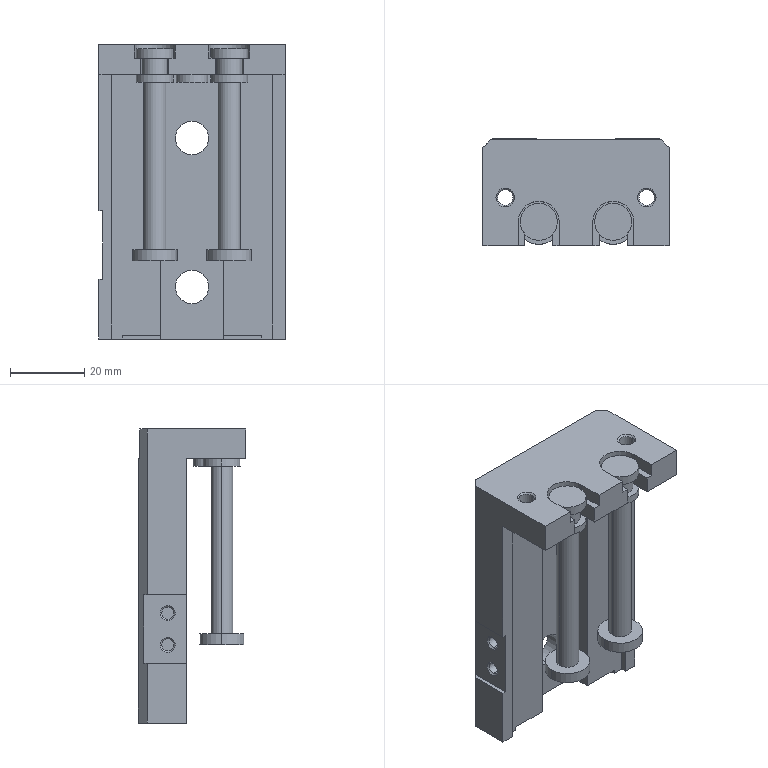Part | SolidWorks | features BaseBody 1 | 1 solid | 174 faces | box 50 x 29 x 79 mm | volume 45333 mm3 | plane 99 | cylinder 59 | cone 16 | commonest cylinder face diameters 3.242 x12 10 x8 4 x5 4.134 x4 4.9 x4 5 x4